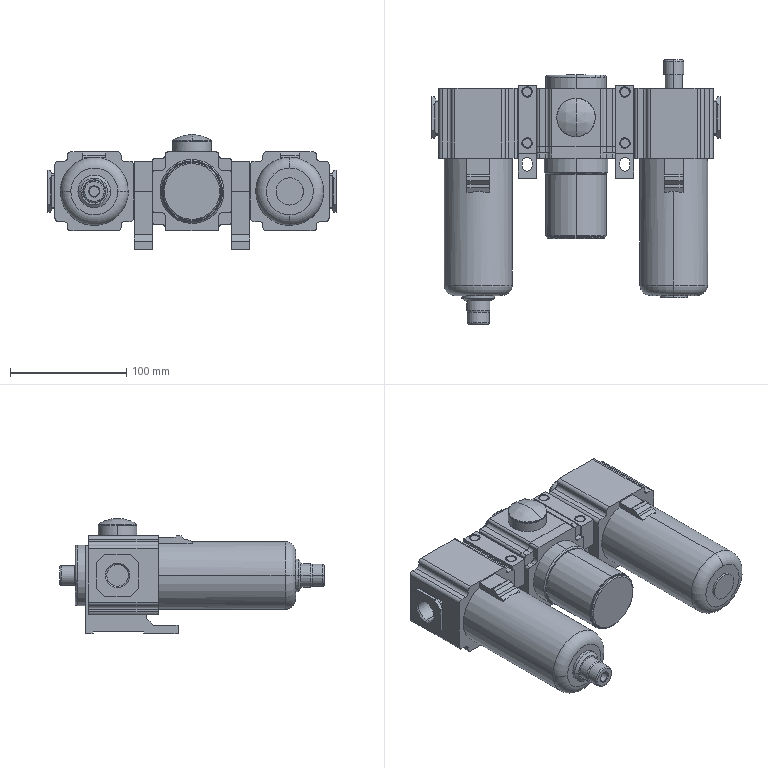Part | SolidWorks | features AEMSimFeature 1 | 5 solids | 466 faces | box 248 x 227 x 99 mm | volume 1707610 mm3 | plane 278 | cylinder 134 | torus 30 | cone 22 | sphere 2 | commonest cylinder face diameters 6 x36 4 x20 18.631 x12 8.5 x8 9 x8 36.2 x8